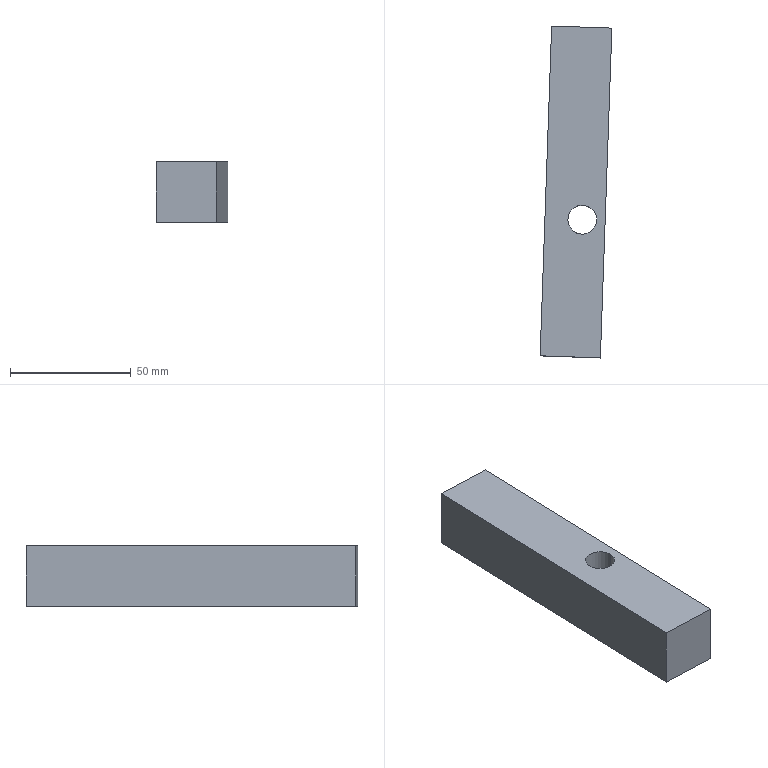Part | STEP file | 1_id1462_x_t | 1 solid | 16 faces | box 29.76 x 137.606 x 25 mm | volume 81885 mm3 | cylinder 6 | plane 6 | cone 4 | commonest cylinder face diameters 5 x4 12 x2
STEP:
#1=CARTESIAN_POINT('',(0.,0.,0.));
#2=DIRECTION('',(0.,0.,1.));
#3=DIRECTION('',(1.,0.,0.));
#4=AXIS2_PLACEMENT_3D('',#1,#2,#3);
#5=CARTESIAN_POINT('',(978.413,154.145,40.46));
#6=VERTEX_POINT('',#5);
#7=CARTESIAN_POINT('',(978.413,154.145,35.46));
#8=VERTEX_POINT('',#7);
#9=CARTESIAN_POINT('',(978.413,154.145,37.96));
#10=DIRECTION('',(0.0349,0.9994,0.));
#11=DIRECTION('',(0.,0.,1.));
#12=AXIS2_PLACEMENT_3D('',#9,#10,#11);
#13=CIRCLE('',#12,2.5);
#14=CARTESIAN_POINT('',(978.389,153.467,37.96));
#15=DIRECTION('',(0.0349,0.9994,0.));
#16=DIRECTION('',(0.,0.,-1.));
#17=AXIS2_PLACEMENT_3D('',#14,#15,#16);
#18=CONICAL_SURFACE('',#17,1.324,1.047);
#19=CARTESIAN_POINT('',(3.142,0.6788));
#20=DIRECTION('',(1.,0.));
#21=VECTOR('',#20,1.);
#22=LINE('',#19,#21);
#23=(GEOMETRIC_REPRESENTATION_CONTEXT(2)PARAMETRIC_REPRESENTATION_CONTEXT()REPRESENTATION_CONTEXT('',''));
#24=DEFINITIONAL_REPRESENTATION('',(#22),#23);
#25=PCURVE('',#18,#24);
#26=CARTESIAN_POINT('',(978.413,154.145,37.96));
#27=DIRECTION('',(-0.0349,-0.9994,0.));
#28=DIRECTION('',(0.,0.,-1.));
#29=AXIS2_PLACEMENT_3D('',#26,#27,#28);
#30=CYLINDRICAL_SURFACE('',#29,2.5);
#31=CARTESIAN_POINT('',(3.142,0.));
#32=DIRECTION('',(-1.,0.));
#33=VECTOR('',#32,1.);
#34=LINE('',#31,#33);
#35=(GEOMETRIC_REPRESENTATION_CONTEXT(2)PARAMETRIC_REPRESENTATION_CONTEXT()REPRESENTATION_CONTEXT('',''));
#36=DEFINITIONAL_REPRESENTATION('',(#34),#35);
#37=PCURVE('',#30,#36);
#38=SURFACE_CURVE('',#13,(#25,#37),.PCURVE_S1.);
#39=EDGE_CURVE('',#6,#8,#38,.T.);
#40=ORIENTED_EDGE('',*,*,#39,.F.);
#41=CARTESIAN_POINT('',(978.362,152.703,37.96));
#42=VERTEX_POINT('',#41);
#43=CARTESIAN_POINT('',(978.362,152.703,37.96));
#44=DIRECTION('',(0.01745,0.4997,0.866));
#45=VECTOR('',#44,1.);
#46=LINE('',#43,#45);
#47=CARTESIAN_POINT('',(3.142,-0.7646));
#48=CARTESIAN_POINT('',(3.142,-0.7427));
#49=CARTESIAN_POINT('',(3.142,-0.699));
#50=CARTESIAN_POINT('',(3.142,-0.6334));
#51=CARTESIAN_POINT('',(3.142,-0.5678));
#52=CARTESIAN_POINT('',(3.142,-0.5022));
#53=CARTESIAN_POINT('',(3.142,-0.4365));
#54=CARTESIAN_POINT('',(3.142,-0.3709));
#55=CARTESIAN_POINT('',(3.142,-0.3053));
#56=CARTESIAN_POINT('',(3.142,-0.2397));
#57=CARTESIAN_POINT('',(3.142,-0.1741));
#58=CARTESIAN_POINT('',(3.142,-0.1085));
#59=CARTESIAN_POINT('',(3.142,-0.0429));
#60=CARTESIAN_POINT('',(3.142,0.02271));
#61=CARTESIAN_POINT('',(3.142,0.08832));
#62=CARTESIAN_POINT('',(3.142,0.1539));
#63=CARTESIAN_POINT('',(3.142,0.2195));
#64=CARTESIAN_POINT('',(3.142,0.2851));
#65=CARTESIAN_POINT('',(3.142,0.3508));
#66=CARTESIAN_POINT('',(3.142,0.4164));
#67=CARTESIAN_POINT('',(3.142,0.482));
#68=CARTESIAN_POINT('',(3.142,0.5476));
#69=CARTESIAN_POINT('',(3.142,0.6132));
#70=CARTESIAN_POINT('',(3.142,0.6569));
#71=CARTESIAN_POINT('',(3.142,0.6788));
#72=B_SPLINE_CURVE_WITH_KNOTS('',3,(#47,#48,#49,#50,#51,#52,#53,#54,#55,#56,#57,#58,#59,#60,#61,#62,#63,#64,#65,#66,#67,#68,#69,#70,#71),.UNSPECIFIED.,.F.,.F.,(4,1,1,1,1,1,1,1,1,1,1,1,1,1,1,1,1,1,1,1,1,1,4),(0.,0.1312,0.2624,0.3936,0.5249,0.6561,0.7873,0.9185,1.05,1.181,1.312,1.443,1.575,1.706,1.837,1.968,2.099,2.231,2.362,2.493,2.624,2.756,2.887),.QUASI_UNIFORM_KNOTS.);
#73=(GEOMETRIC_REPRESENTATION_CONTEXT(2)PARAMETRIC_REPRESENTATION_CONTEXT()REPRESENTATION_CONTEXT('',''));
#74=DEFINITIONAL_REPRESENTATION('',(#72),#73);
#75=PCURVE('',#18,#74);
#76=CARTESIAN_POINT('',(978.389,153.467,37.96));
#77=DIRECTION('',(0.0349,0.9994,0.));
#78=DIRECTION('',(0.,0.,-1.));
#79=AXIS2_PLACEMENT_3D('',#76,#77,#78);
#80=CONICAL_SURFACE('',#79,1.324,1.047);
#81=CARTESIAN_POINT('',(3.142,-0.7646));
#82=CARTESIAN_POINT('',(3.142,-0.7427));
#83=CARTESIAN_POINT('',(3.142,-0.699));
#84=CARTESIAN_POINT('',(3.142,-0.6334));
#85=CARTESIAN_POINT('',(3.142,-0.5678));
#86=CARTESIAN_POINT('',(3.142,-0.5022));
#87=CARTESIAN_POINT('',(3.142,-0.4365));
#88=CARTESIAN_POINT('',(3.142,-0.3709));
#89=CARTESIAN_POINT('',(3.142,-0.3053));
#90=CARTESIAN_POINT('',(3.142,-0.2397));
#91=CARTESIAN_POINT('',(3.142,-0.1741));
#92=CARTESIAN_POINT('',(3.142,-0.1085));
#93=CARTESIAN_POINT('',(3.142,-0.0429));
#94=CARTESIAN_POINT('',(3.142,0.02271));
#95=CARTESIAN_POINT('',(3.142,0.08832));
#96=CARTESIAN_POINT('',(3.142,0.1539));
#97=CARTESIAN_POINT('',(3.142,0.2195));
#98=CARTESIAN_POINT('',(3.142,0.2851));
#99=CARTESIAN_POINT('',(3.142,0.3508));
#100=CARTESIAN_POINT('',(3.142,0.4164));
#101=CARTESIAN_POINT('',(3.142,0.482));
#102=CARTESIAN_POINT('',(3.142,0.5476));
#103=CARTESIAN_POINT('',(3.142,0.6132));
#104=CARTESIAN_POINT('',(3.142,0.6569));
#105=CARTESIAN_POINT('',(3.142,0.6788));
#106=B_SPLINE_CURVE_WITH_KNOTS('',3,(#81,#82,#83,#84,#85,#86,#87,#88,#89,#90,#91,#92,#93,#94,#95,#96,#97,#98,#99,#100,#101,#102,#103,#104,#105),.UNSPECIFIED.,.F.,.F.,(4,1,1,1,1,1,1,1,1,1,1,1,1,1,1,1,1,1,1,1,1,1,4),(0.,0.1312,0.2624,0.3936,0.5249,0.6561,0.7873,0.9185,1.05,1.181,1.312,1.443,1.575,1.706,1.837,1.968,2.099,2.231,2.362,2.493,2.624,2.756,2.887),.QUASI_UNIFORM_KNOTS.);
#107=(GEOMETRIC_REPRESENTATION_CONTEXT(2)PARAMETRIC_REPRESENTATION_CONTEXT()REPRESENTATION_CONTEXT('',''));
#108=DEFINITIONAL_REPRESENTATION('',(#106),#107);
#109=PCURVE('',#80,#108);
#110=SURFACE_CURVE('',#46,(#75,#109),.PCURVE_S1.);
#111=EDGE_CURVE('',#42,#6,#110,.T.);
#112=ORIENTED_EDGE('',*,*,#111,.F.);
#113=CARTESIAN_POINT('',(978.362,152.703,37.96));
#114=DIRECTION('',(-0.01745,-0.4997,0.866));
#115=VECTOR('',#114,1.);
#116=LINE('',#113,#115);
#117=CARTESIAN_POINT('',(6.283,0.6788));
#118=CARTESIAN_POINT('',(6.283,0.6569));
#119=CARTESIAN_POINT('',(6.283,0.6132));
#120=CARTESIAN_POINT('',(6.283,0.5476));
#121=CARTESIAN_POINT('',(6.283,0.482));
#122=CARTESIAN_POINT('',(6.283,0.4164));
#123=CARTESIAN_POINT('',(6.283,0.3508));
#124=CARTESIAN_POINT('',(6.283,0.2851));
#125=CARTESIAN_POINT('',(6.283,0.2195));
#126=CARTESIAN_POINT('',(6.283,0.1539));
#127=CARTESIAN_POINT('',(6.283,0.08832));
#128=CARTESIAN_POINT('',(6.283,0.02271));
#129=CARTESIAN_POINT('',(6.283,-0.0429));
#130=CARTESIAN_POINT('',(6.283,-0.1085));
#131=CARTESIAN_POINT('',(6.283,-0.1741));
#132=CARTESIAN_POINT('',(6.283,-0.2397));
#133=CARTESIAN_POINT('',(6.283,-0.3053));
#134=CARTESIAN_POINT('',(6.283,-0.3709));
#135=CARTESIAN_POINT('',(6.283,-0.4365));
#136=CARTESIAN_POINT('',(6.283,-0.5022));
#137=CARTESIAN_POINT('',(6.283,-0.5678));
#138=CARTESIAN_POINT('',(6.283,-0.6334));
#139=CARTESIAN_POINT('',(6.283,-0.699));
#140=CARTESIAN_POINT('',(6.283,-0.7427));
#141=CARTESIAN_POINT('',(6.283,-0.7646));
#142=B_SPLINE_CURVE_WITH_KNOTS('',3,(#117,#118,#119,#120,#121,#122,#123,#124,#125,#126,#127,#128,#129,#130,#131,#132,#133,#134,#135,#136,#137,#138,#139,#140,#141),.UNSPECIFIED.,.F.,.F.,(4,1,1,1,1,1,1,1,1,1,1,1,1,1,1,1,1,1,1,1,1,1,4),(-2.887,-2.756,-2.624,-2.493,-2.362,-2.231,-2.099,-1.968,-1.837,-1.706,-1.575,-1.443,-1.312,-1.181,-1.05,-0.9185,-0.7873,-0.6561,-0.5249,-0.3936,-0.2624,-0.1312,0.),.QUASI_UNIFORM_KNOTS.);
#143=(GEOMETRIC_REPRESENTATION_CONTEXT(2)PARAMETRIC_REPRESENTATION_CONTEXT()REPRESENTATION_CONTEXT('',''));
#144=DEFINITIONAL_REPRESENTATION('',(#142),#143);
#145=PCURVE('',#18,#144);
#146=CARTESIAN_POINT('',(0.,0.6788));
#147=CARTESIAN_POINT('',(0.,0.6569));
#148=CARTESIAN_POINT('',(0.,0.6132));
#149=CARTESIAN_POINT('',(0.,0.5476));
#150=CARTESIAN_POINT('',(0.,0.482));
#151=CARTESIAN_POINT('',(0.,0.4164));
#152=CARTESIAN_POINT('',(0.,0.3508));
#153=CARTESIAN_POINT('',(0.,0.2851));
#154=CARTESIAN_POINT('',(0.,0.2195));
#155=CARTESIAN_POINT('',(0.,0.1539));
#156=CARTESIAN_POINT('',(0.,0.08832));
#157=CARTESIAN_POINT('',(0.,0.02271));
#158=CARTESIAN_POINT('',(0.,-0.0429));
#159=CARTESIAN_POINT('',(0.,-0.1085));
#160=CARTESIAN_POINT('',(0.,-0.1741));
#161=CARTESIAN_POINT('',(0.,-0.2397));
#162=CARTESIAN_POINT('',(0.,-0.3053));
#163=CARTESIAN_POINT('',(0.,-0.3709));
#164=CARTESIAN_POINT('',(0.,-0.4365));
#165=CARTESIAN_POINT('',(0.,-0.5022));
#166=CARTESIAN_POINT('',(0.,-0.5678));
#167=CARTESIAN_POINT('',(0.,-0.6334));
#168=CARTESIAN_POINT('',(0.,-0.699));
#169=CARTESIAN_POINT('',(0.,-0.7427));
#170=CARTESIAN_POINT('',(0.,-0.7646));
#171=B_SPLINE_CURVE_WITH_KNOTS('',3,(#146,#147,#148,#149,#150,#151,#152,#153,#154,#155,#156,#157,#158,#159,#160,#161,#162,#163,#164,#165,#166,#167,#168,#169,#170),.UNSPECIFIED.,.F.,.F.,(4,1,1,1,1,1,1,1,1,1,1,1,1,1,1,1,1,1,1,1,1,1,4),(-2.887,-2.756,-2.624,-2.493,-2.362,-2.231,-2.099,-1.968,-1.837,-1.706,-1.575,-1.443,-1.312,-1.181,-1.05,-0.9185,-0.7873,-0.6561,-0.5249,-0.3936,-0.2624,-0.1312,0.),.QUASI_UNIFORM_KNOTS.);
#172=(GEOMETRIC_REPRESENTATION_CONTEXT(2)PARAMETRIC_REPRESENTATION_CONTEXT()REPRESENTATION_CONTEXT('',''));
#173=DEFINITIONAL_REPRESENTATION('',(#171),#172);
#174=PCURVE('',#80,#173);
#175=SURFACE_CURVE('',#116,(#145,#174),.PCURVE_S1.);
#176=EDGE_CURVE('',#8,#42,#175,.T.);
#177=ORIENTED_EDGE('',*,*,#176,.F.);
#178=EDGE_LOOP('',(#40,#112,#177));
#179=FACE_BOUND('',#178,.F.);
#180=ADVANCED_FACE('',(#179),#18,.F.);
#181=ORIENTED_EDGE('',*,*,#39,.T.);
#182=CARTESIAN_POINT('',(979.105,173.959,35.46));
#183=VERTEX_POINT('',#182);
#184=CARTESIAN_POINT('',(979.105,173.959,35.46));
#185=DIRECTION('',(0.0349,0.9994,0.));
#186=VECTOR('',#185,1.);
#187=LINE('',#184,#186);
#188=CARTESIAN_POINT('',(0.,-19.826));
#189=DIRECTION('',(0.,-1.));
#190=VECTOR('',#189,1.);
#191=LINE('',#188,#190);
#192=(GEOMETRIC_REPRESENTATION_CONTEXT(2)PARAMETRIC_REPRESENTATION_CONTEXT()REPRESENTATION_CONTEXT('',''));
#193=DEFINITIONAL_REPRESENTATION('',(#191),#192);
#194=PCURVE('',#30,#193);
#195=CARTESIAN_POINT('',(978.413,154.145,37.96));
#196=DIRECTION('',(-0.0349,-0.9994,0.));
#197=DIRECTION('',(0.,0.,-1.));
#198=AXIS2_PLACEMENT_3D('',#195,#196,#197);
#199=CYLINDRICAL_SURFACE('',#198,2.5);
#200=CARTESIAN_POINT('',(6.283,-19.826));
#201=DIRECTION('',(0.,-1.));
#202=VECTOR('',#201,1.);
#203=LINE('',#200,#202);
#204=(GEOMETRIC_REPRESENTATION_CONTEXT(2)PARAMETRIC_REPRESENTATION_CONTEXT()REPRESENTATION_CONTEXT('',''));
#205=DEFINITIONAL_REPRESENTATION('',(#203),#204);
#206=PCURVE('',#199,#205);
#207=SURFACE_CURVE('',#187,(#194,#206),.PCURVE_S1.);
#208=EDGE_CURVE('',#8,#183,#207,.T.);
#209=ORIENTED_EDGE('',*,*,#208,.T.);
#210=CARTESIAN_POINT('',(979.105,173.959,40.46));
#211=VERTEX_POINT('',#210);
#212=CARTESIAN_POINT('',(979.105,173.959,37.96));
#213=DIRECTION('',(-0.0349,-0.9994,0.));
#214=DIRECTION('',(0.,0.,-1.));
#215=AXIS2_PLACEMENT_3D('',#212,#213,#214);
#216=CIRCLE('',#215,2.5);
#217=CARTESIAN_POINT('',(0.,-19.826));
#218=DIRECTION('',(1.,0.));
#219=VECTOR('',#218,1.);
#220=LINE('',#217,#219);
#221=(GEOMETRIC_REPRESENTATION_CONTEXT(2)PARAMETRIC_REPRESENTATION_CONTEXT()REPRESENTATION_CONTEXT('',''));
#222=DEFINITIONAL_REPRESENTATION('',(#220),#221);
#223=PCURVE('',#30,#222);
#224=CARTESIAN_POINT('',(998.241,173.29,9.388));
#225=DIRECTION('',(-0.0349,-0.9994,0.));
#226=DIRECTION('',(0.,0.,1.));
#227=AXIS2_PLACEMENT_3D('',#224,#225,#226);
#228=PLANE('',#227);
#229=CARTESIAN_POINT('',(28.572,19.148));
#230=DIRECTION('',(-1.,0.));
#231=AXIS2_PLACEMENT_2D('',#229,#230);
#232=CIRCLE('',#231,2.5);
#233=(GEOMETRIC_REPRESENTATION_CONTEXT(2)PARAMETRIC_REPRESENTATION_CONTEXT()REPRESENTATION_CONTEXT('',''));
#234=DEFINITIONAL_REPRESENTATION('',(#232),#233);
#235=PCURVE('',#228,#234);
#236=SURFACE_CURVE('',#216,(#223,#235),.PCURVE_S1.);
#237=EDGE_CURVE('',#183,#211,#236,.T.);
#238=ORIENTED_EDGE('',*,*,#237,.T.);
#239=CARTESIAN_POINT('',(979.105,173.959,40.46));
#240=DIRECTION('',(-0.0349,-0.9994,0.));
#241=VECTOR('',#240,1.);
#242=LINE('',#239,#241);
#243=CARTESIAN_POINT('',(3.142,-19.826));
#244=DIRECTION('',(0.,1.));
#245=VECTOR('',#244,1.);
#246=LINE('',#243,#245);
#247=(GEOMETRIC_REPRESENTATION_CONTEXT(2)PARAMETRIC_REPRESENTATION_CONTEXT()REPRESENTATION_CONTEXT('',''));
#248=DEFINITIONAL_REPRESENTATION('',(#246),#247);
#249=PCURVE('',#30,#248);
#250=CARTESIAN_POINT('',(3.142,-19.826));
#251=DIRECTION('',(0.,1.));
#252=VECTOR('',#251,1.);
#253=LINE('',#250,#252);
#254=(GEOMETRIC_REPRESENTATION_CONTEXT(2)PARAMETRIC_REPRESENTATION_CONTEXT()REPRESENTATION_CONTEXT('',''));
#255=DEFINITIONAL_REPRESENTATION('',(#253),#254);
#256=PCURVE('',#199,#255);
#257=SURFACE_CURVE('',#242,(#249,#256),.PCURVE_S1.);
#258=EDGE_CURVE('',#211,#6,#257,.T.);
#259=ORIENTED_EDGE('',*,*,#258,.T.);
#260=EDGE_LOOP('',(#181,#209,#238,#259));
#261=FACE_BOUND('',#260,.F.);
#262=ADVANCED_FACE('',(#261),#30,.F.);
#263=CARTESIAN_POINT('',(978.413,154.145,37.96));
#264=DIRECTION('',(0.0349,0.9994,0.));
#265=DIRECTION('',(0.,0.,-1.));
#266=AXIS2_PLACEMENT_3D('',#263,#264,#265);
#267=CIRCLE('',#266,2.5);
#268=CARTESIAN_POINT('',(6.283,0.));
#269=DIRECTION('',(-1.,0.));
#270=VECTOR('',#269,1.);
#271=LINE('',#268,#270);
#272=(GEOMETRIC_REPRESENTATION_CONTEXT(2)PARAMETRIC_REPRESENTATION_CONTEXT()REPRESENTATION_CONTEXT('',''));
#273=DEFINITIONAL_REPRESENTATION('',(#271),#272);
#274=PCURVE('',#199,#273);
#275=CARTESIAN_POINT('',(0.,0.6788));
#276=DIRECTION('',(1.,0.));
#277=VECTOR('',#276,1.);
#278=LINE('',#275,#277);
#279=(GEOMETRIC_REPRESENTATION_CONTEXT(2)PARAMETRIC_REPRESENTATION_CONTEXT()REPRESENTATION_CONTEXT('',''));
#280=DEFINITIONAL_REPRESENTATION('',(#278),#279);
#281=PCURVE('',#80,#280);
#282=SURFACE_CURVE('',#267,(#274,#281),.PCURVE_S1.);
#283=EDGE_CURVE('',#8,#6,#282,.T.);
#284=ORIENTED_EDGE('',*,*,#283,.T.);
#285=ORIENTED_EDGE('',*,*,#258,.F.);
#286=CARTESIAN_POINT('',(976.606,174.046,37.96));
#287=VERTEX_POINT('',#286);
#288=CARTESIAN_POINT('',(979.105,173.959,37.96));
#289=DIRECTION('',(-0.0349,-0.9994,0.));
#290=DIRECTION('',(0.,0.,1.));
#291=AXIS2_PLACEMENT_3D('',#288,#289,#290);
#292=CIRCLE('',#291,2.5);
#293=CARTESIAN_POINT('',(3.142,-19.826));
#294=DIRECTION('',(1.,0.));
#295=VECTOR('',#294,1.);
#296=LINE('',#293,#295);
#297=(GEOMETRIC_REPRESENTATION_CONTEXT(2)PARAMETRIC_REPRESENTATION_CONTEXT()REPRESENTATION_CONTEXT('',''));
#298=DEFINITIONAL_REPRESENTATION('',(#296),#297);
#299=PCURVE('',#199,#298);
#300=CARTESIAN_POINT('',(28.572,19.148));
#301=DIRECTION('',(1.,0.));
#302=AXIS2_PLACEMENT_2D('',#300,#301);
#303=CIRCLE('',#302,2.5);
#304=(GEOMETRIC_REPRESENTATION_CONTEXT(2)PARAMETRIC_REPRESENTATION_CONTEXT()REPRESENTATION_CONTEXT('',''));
#305=DEFINITIONAL_REPRESENTATION('',(#303),#304);
#306=PCURVE('',#228,#305);
#307=SURFACE_CURVE('',#292,(#299,#306),.PCURVE_S1.);
#308=EDGE_CURVE('',#211,#287,#307,.T.);
#309=ORIENTED_EDGE('',*,*,#308,.T.);
#310=CARTESIAN_POINT('',(979.105,173.959,37.96));
#311=DIRECTION('',(-0.0349,-0.9994,0.));
#312=DIRECTION('',(-0.9994,0.0349,0.));
#313=AXIS2_PLACEMENT_3D('',#310,#311,#312);
#314=CIRCLE('',#313,2.5);
#315=CARTESIAN_POINT('',(4.712,-19.826));
#316=DIRECTION('',(1.,0.));
#317=VECTOR('',#316,1.);
#318=LINE('',#315,#317);
#319=(GEOMETRIC_REPRESENTATION_CONTEXT(2)PARAMETRIC_REPRESENTATION_CONTEXT()REPRESENTATION_CONTEXT('',''));
#320=DEFINITIONAL_REPRESENTATION('',(#318),#319);
#321=PCURVE('',#199,#320);
#322=CARTESIAN_POINT('',(28.572,19.148));
#323=DIRECTION('',(0.,1.));
#324=AXIS2_PLACEMENT_2D('',#322,#323);
#325=CIRCLE('',#324,2.5);
#326=(GEOMETRIC_REPRESENTATION_CONTEXT(2)PARAMETRIC_REPRESENTATION_CONTEXT()REPRESENTATION_CONTEXT('',''));
#327=DEFINITIONAL_REPRESENTATION('',(#325),#326);
#328=PCURVE('',#228,#327);
#329=SURFACE_CURVE('',#314,(#321,#328),.PCURVE_S1.);
#330=EDGE_CURVE('',#287,#183,#329,.T.);
#331=ORIENTED_EDGE('',*,*,#330,.T.);
#332=ORIENTED_EDGE('',*,*,#208,.F.);
#333=EDGE_LOOP('',(#284,#285,#309,#331,#332));
#334=FACE_BOUND('',#333,.F.);
#335=ADVANCED_FACE('',(#334),#199,.F.);
#336=ORIENTED_EDGE('',*,*,#283,.F.);
#337=ORIENTED_EDGE('',*,*,#176,.T.);
#338=ORIENTED_EDGE('',*,*,#111,.T.);
#339=EDGE_LOOP('',(#336,#337,#338));
#340=FACE_BOUND('',#339,.F.);
#341=ADVANCED_FACE('',(#340),#80,.F.);
#342=CARTESIAN_POINT('',(994.092,173.435,43.96));
#343=VERTEX_POINT('',#342);
#344=CARTESIAN_POINT('',(994.092,173.435,18.96));
#345=VERTEX_POINT('',#344);
#346=CARTESIAN_POINT('',(994.092,173.435,43.96));
#347=DIRECTION('',(0.,0.,-1.));
#348=VECTOR('',#347,1.);
#349=LINE('',#346,#348);
#350=CARTESIAN_POINT('',(34.572,4.151));
#351=DIRECTION('',(-1.,0.));
#352=VECTOR('',#351,1.);
#353=LINE('',#350,#352);
#354=(GEOMETRIC_REPRESENTATION_CONTEXT(2)PARAMETRIC_REPRESENTATION_CONTEXT()REPRESENTATION_CONTEXT('',''));
#355=DEFINITIONAL_REPRESENTATION('',(#353),#354);
#356=PCURVE('',#228,#355);
#357=CARTESIAN_POINT('',(994.029,171.611,28.96));
#358=DIRECTION('',(0.9994,-0.0349,0.));
#359=DIRECTION('',(-0.0349,-0.9994,0.));
#360=AXIS2_PLACEMENT_3D('',#357,#358,#359);
#361=PLANE('',#360);
#362=CARTESIAN_POINT('',(-1.826,-15.));
#363=DIRECTION('',(0.,1.));
#364=VECTOR('',#363,1.);
#365=LINE('',#362,#364);
#366=(GEOMETRIC_REPRESENTATION_CONTEXT(2)PARAMETRIC_REPRESENTATION_CONTEXT()REPRESENTATION_CONTEXT('',''));
#367=DEFINITIONAL_REPRESENTATION('',(#365),#366);
#368=PCURVE('',#361,#367);
#369=SURFACE_CURVE('',#349,(#356,#368),.PCURVE_S1.);
#370=EDGE_CURVE('',#343,#345,#369,.T.);
#371=ORIENTED_EDGE('',*,*,#370,.T.);
#372=CARTESIAN_POINT('',(969.108,174.308,18.96));
#373=VERTEX_POINT('',#372);
#374=CARTESIAN_POINT('',(969.108,174.308,18.96));
#375=DIRECTION('',(0.9994,-0.0349,0.));
#376=VECTOR('',#375,1.);
#377=LINE('',#374,#376);
#378=CARTESIAN_POINT('',(9.572,29.151));
#379=DIRECTION('',(0.,-1.));
#380=VECTOR('',#379,1.);
#381=LINE('',#378,#380);
#382=(GEOMETRIC_REPRESENTATION_CONTEXT(2)PARAMETRIC_REPRESENTATION_CONTEXT()REPRESENTATION_CONTEXT('',''));
#383=DEFINITIONAL_REPRESENTATION('',(#381),#382);
#384=PCURVE('',#228,#383);
#385=CARTESIAN_POINT('',(988.334,151.797,18.96));
#386=DIRECTION('',(0.,0.,1.));
#387=DIRECTION('',(1.,0.,0.));
#388=AXIS2_PLACEMENT_3D('',#385,#386,#387);
#389=PLANE('',#388);
#390=CARTESIAN_POINT('',(-19.226,22.51));
#391=DIRECTION('',(0.9994,-0.0349));
#392=VECTOR('',#391,1.);
#393=LINE('',#390,#392);
#394=(GEOMETRIC_REPRESENTATION_CONTEXT(2)PARAMETRIC_REPRESENTATION_CONTEXT()REPRESENTATION_CONTEXT('',''));
#395=DEFINITIONAL_REPRESENTATION('',(#393),#394);
#396=PCURVE('',#389,#395);
#397=SURFACE_CURVE('',#377,(#384,#396),.PCURVE_S1.);
#398=EDGE_CURVE('',#373,#345,#397,.T.);
#399=ORIENTED_EDGE('',*,*,#398,.F.);
#400=CARTESIAN_POINT('',(969.108,174.308,43.96));
#401=VERTEX_POINT('',#400);
#402=CARTESIAN_POINT('',(969.108,174.308,43.96));
#403=DIRECTION('',(0.,0.,-1.));
#404=VECTOR('',#403,1.);
#405=LINE('',#402,#404);
#406=CARTESIAN_POINT('',(34.572,29.151));
#407=DIRECTION('',(-1.,0.));
#408=VECTOR('',#407,1.);
#409=LINE('',#406,#408);
#410=(GEOMETRIC_REPRESENTATION_CONTEXT(2)PARAMETRIC_REPRESENTATION_CONTEXT()REPRESENTATION_CONTEXT('',''));
#411=DEFINITIONAL_REPRESENTATION('',(#409),#410);
#412=PCURVE('',#228,#411);
#413=CARTESIAN_POINT('',(968.346,152.495,28.96));
#414=DIRECTION('',(-0.9994,0.0349,0.));
#415=DIRECTION('',(0.,0.,1.));
#416=AXIS2_PLACEMENT_3D('',#413,#414,#415);
#417=PLANE('',#416);
#418=CARTESIAN_POINT('',(15.,21.826));
#419=DIRECTION('',(-1.,0.));
#420=VECTOR('',#419,1.);
#421=LINE('',#418,#420);
#422=(GEOMETRIC_REPRESENTATION_CONTEXT(2)PARAMETRIC_REPRESENTATION_CONTEXT()REPRESENTATION_CONTEXT('',''));
#423=DEFINITIONAL_REPRESENTATION('',(#421),#422);
#424=PCURVE('',#417,#423);
#425=SURFACE_CURVE('',#405,(#412,#424),.PCURVE_S1.);
#426=EDGE_CURVE('',#401,#373,#425,.T.);
#427=ORIENTED_EDGE('',*,*,#426,.F.);
#428=CARTESIAN_POINT('',(994.092,173.435,43.96));
#429=DIRECTION('',(-0.9994,0.0349,0.));
#430=VECTOR('',#429,1.);
#431=LINE('',#428,#430);
#432=CARTESIAN_POINT('',(34.572,4.151));
#433=DIRECTION('',(0.,1.));
#434=VECTOR('',#433,1.);
#435=LINE('',#432,#434);
#436=(GEOMETRIC_REPRESENTATION_CONTEXT(2)PARAMETRIC_REPRESENTATION_CONTEXT()REPRESENTATION_CONTEXT('',''));
#437=DEFINITIONAL_REPRESENTATION('',(#435),#436);
#438=PCURVE('',#228,#437);
#439=CARTESIAN_POINT('',(988.334,151.797,43.96));
#440=DIRECTION('',(0.,0.,1.));
#441=DIRECTION('',(1.,0.,0.));
#442=AXIS2_PLACEMENT_3D('',#439,#440,#441);
#443=PLANE('',#442);
#444=CARTESIAN_POINT('',(5.759,21.638));
#445=DIRECTION('',(-0.9994,0.0349));
#446=VECTOR('',#445,1.);
#447=LINE('',#444,#446);
#448=(GEOMETRIC_REPRESENTATION_CONTEXT(2)PARAMETRIC_REPRESENTATION_CONTEXT()REPRESENTATION_CONTEXT('',''));
#449=DEFINITIONAL_REPRESENTATION('',(#447),#448);
#450=PCURVE('',#443,#449);
#451=SURFACE_CURVE('',#431,(#438,#450),.PCURVE_S1.);
#452=EDGE_CURVE('',#343,#401,#451,.T.);
#453=ORIENTED_EDGE('',*,*,#452,.F.);
#454=EDGE_LOOP('',(#371,#399,#427,#453));
#455=FACE_BOUND('',#454,.T.);
#456=ORIENTED_EDGE('',*,*,#237,.T.);
#457=ORIENTED_EDGE('',*,*,#308,.T.);
#458=ORIENTED_EDGE('',*,*,#330,.T.);
#459=EDGE_LOOP('',(#456,#457,#458));
#460=FACE_BOUND('',#459,.T.);
#461=CARTESIAN_POINT('',(979.105,173.959,22.46));
#462=VERTEX_POINT('',#461);
#463=CARTESIAN_POINT('',(979.105,173.959,27.46));
#464=VERTEX_POINT('',#463);
#465=CARTESIAN_POINT('',(979.105,173.959,24.96));
#466=DIRECTION('',(-0.0349,-0.9994,0.));
#467=DIRECTION('',(0.,0.,-1.));
#468=AXIS2_PLACEMENT_3D('',#465,#466,#467);
#469=CIRCLE('',#468,2.5);
#470=CARTESIAN_POINT('',(15.572,19.148));
#471=DIRECTION('',(-1.,0.));
#472=AXIS2_PLACEMENT_2D('',#470,#471);
#473=CIRCLE('',#472,2.5);
#474=(GEOMETRIC_REPRESENTATION_CONTEXT(2)PARAMETRIC_REPRESENTATION_CONTEXT()REPRESENTATION_CONTEXT('',''));
#475=DEFINITIONAL_REPRESENTATION('',(#473),#474);
#476=PCURVE('',#228,#475);
#477=CARTESIAN_POINT('',(978.413,154.145,24.96));
#478=DIRECTION('',(-0.0349,-0.9994,0.));
#479=DIRECTION('',(0.,0.,-1.));
#480=AXIS2_PLACEMENT_3D('',#477,#478,#479);
#481=CYLINDRICAL_SURFACE('',#480,2.5);
#482=CARTESIAN_POINT('',(0.,-19.826));
#483=DIRECTION('',(1.,0.));
#484=VECTOR('',#483,1.);
#485=LINE('',#482,#484);
#486=(GEOMETRIC_REPRESENTATION_CONTEXT(2)PARAMETRIC_REPRESENTATION_CONTEXT()REPRESENTATION_CONTEXT('',''));
#487=DEFINITIONAL_REPRESENTATION('',(#485),#486);
#488=PCURVE('',#481,#487);
#489=SURFACE_CURVE('',#469,(#476,#488),.PCURVE_S1.);
#490=EDGE_CURVE('',#462,#464,#489,.T.);
#491=ORIENTED_EDGE('',*,*,#490,.T.);
#492=CARTESIAN_POINT('',(976.606,174.046,24.96));
#493=VERTEX_POINT('',#492);
#494=CARTESIAN_POINT('',(979.105,173.959,24.96));
#495=DIRECTION('',(-0.0349,-0.9994,0.));
#496=DIRECTION('',(0.,0.,1.));
#497=AXIS2_PLACEMENT_3D('',#494,#495,#496);
#498=CIRCLE('',#497,2.5);
#499=CARTESIAN_POINT('',(15.572,19.148));
#500=DIRECTION('',(1.,0.));
#501=AXIS2_PLACEMENT_2D('',#499,#500);
#502=CIRCLE('',#501,2.5);
#503=(GEOMETRIC_REPRESENTATION_CONTEXT(2)PARAMETRIC_REPRESENTATION_CONTEXT()REPRESENTATION_CONTEXT('',''));
#504=DEFINITIONAL_REPRESENTATION('',(#502),#503);
#505=PCURVE('',#228,#504);
#506=CARTESIAN_POINT('',(978.413,154.145,24.96));
#507=DIRECTION('',(-0.0349,-0.9994,0.));
#508=DIRECTION('',(0.,0.,-1.));
#509=AXIS2_PLACEMENT_3D('',#506,#507,#508);
#510=CYLINDRICAL_SURFACE('',#509,2.5);
#511=CARTESIAN_POINT('',(3.142,-19.826));
#512=DIRECTION('',(1.,0.));
#513=VECTOR('',#512,1.);
#514=LINE('',#511,#513);
#515=(GEOMETRIC_REPRESENTATION_CONTEXT(2)PARAMETRIC_REPRESENTATION_CONTEXT()REPRESENTATION_CONTEXT('',''));
#516=DEFINITIONAL_REPRESENTATION('',(#514),#515);
#517=PCURVE('',#510,#516);
#518=SURFACE_CURVE('',#498,(#505,#517),.PCURVE_S1.);
#519=EDGE_CURVE('',#464,#493,#518,.T.);
#520=ORIENTED_EDGE('',*,*,#519,.T.);
#521=CARTESIAN_POINT('',(979.105,173.959,24.96));
#522=DIRECTION('',(-0.0349,-0.9994,0.));
#523=DIRECTION('',(-0.9994,0.0349,0.));
#524=AXIS2_PLACEMENT_3D('',#521,#522,#523);
#525=CIRCLE('',#524,2.5);
#526=CARTESIAN_POINT('',(15.572,19.148));
#527=DIRECTION('',(0.,1.));
#528=AXIS2_PLACEMENT_2D('',#526,#527);
#529=CIRCLE('',#528,2.5);
#530=(GEOMETRIC_REPRESENTATION_CONTEXT(2)PARAMETRIC_REPRESENTATION_CONTEXT()REPRESENTATION_CONTEXT('',''));
#531=DEFINITIONAL_REPRESENTATION('',(#529),#530);
#532=PCURVE('',#228,#531);
#533=CARTESIAN_POINT('',(4.712,-19.826));
#534=DIRECTION('',(1.,0.));
#535=VECTOR('',#534,1.);
#536=LINE('',#533,#535);
#537=(GEOMETRIC_REPRESENTATION_CONTEXT(2)PARAMETRIC_REPRESENTATION_CONTEXT()REPRESENTATION_CONTEXT('',''));
#538=DEFINITIONAL_REPRESENTATION('',(#536),#537);
#539=PCURVE('',#510,#538);
#540=SURFACE_CURVE('',#525,(#532,#539),.PCURVE_S1.);
#541=EDGE_CURVE('',#493,#462,#540,.T.);
#542=ORIENTED_EDGE('',*,*,#541,.T.);
#543=EDGE_LOOP('',(#491,#520,#542));
#544=FACE_BOUND('',#543,.T.);
#545=ADVANCED_FACE('',(#455,#460,#544),#228,.F.);
#546=CARTESIAN_POINT('',(964.333,37.575,43.96));
#547=VERTEX_POINT('',#546);
#548=CARTESIAN_POINT('',(989.318,36.702,43.96));
#549=VERTEX_POINT('',#548);
#550=CARTESIAN_POINT('',(964.333,37.575,43.96));
#551=DIRECTION('',(0.9994,-0.0349,0.));
#552=VECTOR('',#551,1.);
#553=LINE('',#550,#552);
#554=CARTESIAN_POINT('',(-24.001,-114.223));
#555=DIRECTION('',(0.9994,-0.0349));
#556=VECTOR('',#555,1.);
#557=LINE('',#554,#556);
#558=(GEOMETRIC_REPRESENTATION_CONTEXT(2)PARAMETRIC_REPRESENTATION_CONTEXT()REPRESENTATION_CONTEXT('',''));
#559=DEFINITIONAL_REPRESENTATION('',(#557),#558);
#560=PCURVE('',#443,#559);
#561=CARTESIAN_POINT('',(984.844,36.858,28.96));
#562=DIRECTION('',(-0.0349,-0.9994,0.));
#563=DIRECTION('',(0.,0.,1.));
#564=AXIS2_PLACEMENT_3D('',#561,#562,#563);
#565=PLANE('',#564);
#566=CARTESIAN_POINT('',(15.,20.523));
#567=DIRECTION('',(0.,-1.));
#568=VECTOR('',#567,1.);
#569=LINE('',#566,#568);
#570=(GEOMETRIC_REPRESENTATION_CONTEXT(2)PARAMETRIC_REPRESENTATION_CONTEXT()REPRESENTATION_CONTEXT('',''));
#571=DEFINITIONAL_REPRESENTATION('',(#569),#570);
#572=PCURVE('',#565,#571);
#573=SURFACE_CURVE('',#553,(#560,#572),.PCURVE_S1.);
#574=EDGE_CURVE('',#547,#549,#573,.T.);
#575=ORIENTED_EDGE('',*,*,#574,.T.);
#576=CARTESIAN_POINT('',(989.318,36.702,43.96));
#577=DIRECTION('',(0.0349,0.9994,0.));
#578=VECTOR('',#577,1.);
#579=LINE('',#576,#578);
#580=CARTESIAN_POINT('',(0.9838,-115.095));
#581=DIRECTION('',(0.0349,0.9994));
#582=VECTOR('',#581,1.);
#583=LINE('',#580,#582);
#584=(GEOMETRIC_REPRESENTATION_CONTEXT(2)PARAMETRIC_REPRESENTATION_CONTEXT()REPRESENTATION_CONTEXT('',''));
#585=DEFINITIONAL_REPRESENTATION('',(#583),#584);
#586=PCURVE('',#443,#585);
#587=CARTESIAN_POINT('',(134.991,-15.));
#588=DIRECTION('',(-1.,0.));
#589=VECTOR('',#588,1.);
#590=LINE('',#587,#589);
#591=(GEOMETRIC_REPRESENTATION_CONTEXT(2)PARAMETRIC_REPRESENTATION_CONTEXT()REPRESENTATION_CONTEXT('',''));
#592=DEFINITIONAL_REPRESENTATION('',(#590),#591);
#593=PCURVE('',#361,#592);
#594=SURFACE_CURVE('',#579,(#586,#593),.PCURVE_S1.);
#595=EDGE_CURVE('',#549,#343,#594,.T.);
#596=ORIENTED_EDGE('',*,*,#595,.T.);
#597=ORIENTED_EDGE('',*,*,#452,.T.);
#598=CARTESIAN_POINT('',(969.108,174.308,43.96));
#599=DIRECTION('',(-0.0349,-0.9994,0.));
#600=VECTOR('',#599,1.);
#601=LINE('',#598,#600);
#602=CARTESIAN_POINT('',(-19.226,22.51));
#603=DIRECTION('',(-0.0349,-0.9994));
#604=VECTOR('',#603,1.);
#605=LINE('',#602,#604);
#606=(GEOMETRIC_REPRESENTATION_CONTEXT(2)PARAMETRIC_REPRESENTATION_CONTEXT()REPRESENTATION_CONTEXT('',''));
#607=DEFINITIONAL_REPRESENTATION('',(#605),#606);
#608=PCURVE('',#443,#607);
#609=CARTESIAN_POINT('',(15.,21.826));
#610=DIRECTION('',(0.,-1.));
#611=VECTOR('',#610,1.);
#612=LINE('',#609,#611);
#613=(GEOMETRIC_REPRESENTATION_CONTEXT(2)PARAMETRIC_REPRESENTATION_CONTEXT()REPRESENTATION_CONTEXT('',''));
#614=DEFINITIONAL_REPRESENTATION('',(#612),#613);
#615=PCURVE('',#417,#614);
#616=SURFACE_CURVE('',#601,(#608,#615),.PCURVE_S1.);
#617=EDGE_CURVE('',#401,#547,#616,.T.);
#618=ORIENTED_EDGE('',*,*,#617,.T.);
#619=EDGE_LOOP('',(#575,#596,#597,#618));
#620=FACE_BOUND('',#619,.T.);
#621=CARTESIAN_POINT('',(987.832,93.789,43.96));
#622=VERTEX_POINT('',#621);
#623=CARTESIAN_POINT('',(975.84,94.208,43.96));
#624=VERTEX_POINT('',#623);
#625=CARTESIAN_POINT('',(981.836,93.998,43.96));
#626=DIRECTION('',(0.,0.,-1.));
#627=DIRECTION('',(0.9994,-0.0349,0.));
#628=AXIS2_PLACEMENT_3D('',#625,#626,#627);
#629=CIRCLE('',#628,6.);
#630=CARTESIAN_POINT('',(-0.5013,-58.009));
#631=CARTESIAN_POINT('',(-0.864,-68.395));
#632=CARTESIAN_POINT('',(-9.677,-62.888));
#633=CARTESIAN_POINT('',(-18.49,-57.381));
#634=CARTESIAN_POINT('',(-9.314,-52.502));
#635=CARTESIAN_POINT('',(-0.1386,-47.623));
#636=CARTESIAN_POINT('',(-0.5013,-58.009));
#637=(BOUNDED_CURVE()B_SPLINE_CURVE(2,(#630,#631,#632,#633,#634,#635,#636),.UNSPECIFIED.,.T.,.F.)B_SPLINE_CURVE_WITH_KNOTS((1,2,2,2,2,1),(-2.094,0.,2.094,4.189,6.283,8.378),.UNSPECIFIED.)CURVE()GEOMETRIC_REPRESENTATION_ITEM()RATIONAL_B_SPLINE_CURVE((1.,0.5,1.,0.5,1.,0.5,1.))REPRESENTATION_ITEM(''));
#638=(GEOMETRIC_REPRESENTATION_CONTEXT(2)PARAMETRIC_REPRESENTATION_CONTEXT()REPRESENTATION_CONTEXT('',''));
#639=DEFINITIONAL_REPRESENTATION('',(#637),#638);
#640=PCURVE('',#443,#639);
#641=CARTESIAN_POINT('',(981.836,93.998,12.96));
#642=DIRECTION('',(0.,0.,-1.));
#643=DIRECTION('',(0.9994,-0.0349,0.));
#644=AXIS2_PLACEMENT_3D('',#641,#642,#643);
#645=CYLINDRICAL_SURFACE('',#644,6.);
#646=CARTESIAN_POINT('',(0.,-31.));
#647=DIRECTION('',(1.,0.));
#648=VECTOR('',#647,1.);
#649=LINE('',#646,#648);
#650=(GEOMETRIC_REPRESENTATION_CONTEXT(2)PARAMETRIC_REPRESENTATION_CONTEXT()REPRESENTATION_CONTEXT('',''));
#651=DEFINITIONAL_REPRESENTATION('',(#649),#650);
#652=PCURVE('',#645,#651);
#653=SURFACE_CURVE('',#629,(#640,#652),.PCURVE_S1.);
#654=EDGE_CURVE('',#622,#624,#653,.T.);
#655=ORIENTED_EDGE('',*,*,#654,.T.);
#656=CARTESIAN_POINT('',(981.836,93.998,43.96));
#657=DIRECTION('',(0.,0.,-1.));
#658=DIRECTION('',(-0.9994,0.0349,0.));
#659=AXIS2_PLACEMENT_3D('',#656,#657,#658);
#660=CIRCLE('',#659,6.);
#661=CARTESIAN_POINT('',(-12.494,-57.59));
#662=CARTESIAN_POINT('',(-12.131,-47.204));
#663=CARTESIAN_POINT('',(-3.318,-52.711));
#664=CARTESIAN_POINT('',(5.495,-58.218));
#665=CARTESIAN_POINT('',(-3.681,-63.097));
#666=CARTESIAN_POINT('',(-12.857,-67.976));
#667=CARTESIAN_POINT('',(-12.494,-57.59));
#668=(BOUNDED_CURVE()B_SPLINE_CURVE(2,(#661,#662,#663,#664,#665,#666,#667),.UNSPECIFIED.,.T.,.F.)B_SPLINE_CURVE_WITH_KNOTS((1,2,2,2,2,1),(-2.094,0.,2.094,4.189,6.283,8.378),.UNSPECIFIED.)CURVE()GEOMETRIC_REPRESENTATION_ITEM()RATIONAL_B_SPLINE_CURVE((1.,0.5,1.,0.5,1.,0.5,1.))REPRESENTATION_ITEM(''));
#669=(GEOMETRIC_REPRESENTATION_CONTEXT(2)PARAMETRIC_REPRESENTATION_CONTEXT()REPRESENTATION_CONTEXT('',''));
#670=DEFINITIONAL_REPRESENTATION('',(#668),#669);
#671=PCURVE('',#443,#670);
#672=CARTESIAN_POINT('',(981.836,93.998,12.96));
#673=DIRECTION('',(0.,0.,-1.));
#674=DIRECTION('',(0.9994,-0.0349,0.));
#675=AXIS2_PLACEMENT_3D('',#672,#673,#674);
#676=CYLINDRICAL_SURFACE('',#675,6.);
#677=CARTESIAN_POINT('',(3.142,-31.));
#678=DIRECTION('',(1.,0.));
#679=VECTOR('',#678,1.);
#680=LINE('',#677,#679);
#681=(GEOMETRIC_REPRESENTATION_CONTEXT(2)PARAMETRIC_REPRESENTATION_CONTEXT()REPRESENTATION_CONTEXT('',''));
#682=DEFINITIONAL_REPRESENTATION('',(#680),#681);
#683=PCURVE('',#676,#682);
#684=SURFACE_CURVE('',#660,(#671,#683),.PCURVE_S1.);
#685=EDGE_CURVE('',#624,#622,#684,.T.);
#686=ORIENTED_EDGE('',*,*,#685,.T.);
#687=EDGE_LOOP('',(#655,#686));
#688=FACE_BOUND('',#687,.T.);
#689=ADVANCED_FACE('',(#620,#688),#443,.T.);
#690=ORIENTED_EDGE('',*,*,#617,.F.);
#691=ORIENTED_EDGE('',*,*,#426,.T.);
#692=CARTESIAN_POINT('',(964.333,37.575,18.96));
#693=VERTEX_POINT('',#692);
#694=CARTESIAN_POINT('',(964.333,37.575,18.96));
#695=DIRECTION('',(0.0349,0.9994,0.));
#696=VECTOR('',#695,1.);
#697=LINE('',#694,#696);
#698=CARTESIAN_POINT('',(-10.,-114.991));
#699=DIRECTION('',(0.,1.));
#700=VECTOR('',#699,1.);
#701=LINE('',#698,#700);
#702=(GEOMETRIC_REPRESENTATION_CONTEXT(2)PARAMETRIC_REPRESENTATION_CONTEXT()REPRESENTATION_CONTEXT('',''));
#703=DEFINITIONAL_REPRESENTATION('',(#701),#702);
#704=PCURVE('',#417,#703);
#705=CARTESIAN_POINT('',(-24.001,-114.223));
#706=DIRECTION('',(0.0349,0.9994));
#707=VECTOR('',#706,1.);
#708=LINE('',#705,#707);
#709=(GEOMETRIC_REPRESENTATION_CONTEXT(2)PARAMETRIC_REPRESENTATION_CONTEXT()REPRESENTATION_CONTEXT('',''));
#710=DEFINITIONAL_REPRESENTATION('',(#708),#709);
#711=PCURVE('',#389,#710);
#712=SURFACE_CURVE('',#697,(#704,#711),.PCURVE_S1.);
#713=EDGE_CURVE('',#693,#373,#712,.T.);
#714=ORIENTED_EDGE('',*,*,#713,.F.);
#715=CARTESIAN_POINT('',(964.333,37.575,43.96));
#716=DIRECTION('',(0.,0.,-1.));
#717=VECTOR('',#716,1.);
#718=LINE('',#715,#717);
#719=CARTESIAN_POINT('',(15.,-114.991));
#720=DIRECTION('',(-1.,0.));
#721=VECTOR('',#720,1.);
#722=LINE('',#719,#721);
#723=(GEOMETRIC_REPRESENTATION_CONTEXT(2)PARAMETRIC_REPRESENTATION_CONTEXT()REPRESENTATION_CONTEXT('',''));
#724=DEFINITIONAL_REPRESENTATION('',(#722),#723);
#725=PCURVE('',#417,#724);
#726=CARTESIAN_POINT('',(15.,20.523));
#727=DIRECTION('',(-1.,0.));
#728=VECTOR('',#727,1.);
#729=LINE('',#726,#728);
#730=(GEOMETRIC_REPRESENTATION_CONTEXT(2)PARAMETRIC_REPRESENTATION_CONTEXT()REPRESENTATION_CONTEXT('',''));
#731=DEFINITIONAL_REPRESENTATION('',(#729),#730);
#732=PCURVE('',#565,#731);
#733=SURFACE_CURVE('',#718,(#725,#732),.PCURVE_S1.);
#734=EDGE_CURVE('',#547,#693,#733,.T.);
#735=ORIENTED_EDGE('',*,*,#734,.F.);
#736=EDGE_LOOP('',(#690,#691,#714,#735));
#737=FACE_BOUND('',#736,.T.);
#738=ADVANCED_FACE('',(#737),#417,.T.);
#739=ORIENTED_EDGE('',*,*,#574,.F.);
#740=ORIENTED_EDGE('',*,*,#734,.T.);
#741=CARTESIAN_POINT('',(989.318,36.702,18.96));
#742=VERTEX_POINT('',#741);
#743=CARTESIAN_POINT('',(989.318,36.702,18.96));
#744=DIRECTION('',(-0.9994,0.0349,0.));
#745=VECTOR('',#744,1.);
#746=LINE('',#743,#745);
#747=CARTESIAN_POINT('',(-10.,-4.477));
#748=DIRECTION('',(0.,1.));
#749=VECTOR('',#748,1.);
#750=LINE('',#747,#749);
#751=(GEOMETRIC_REPRESENTATION_CONTEXT(2)PARAMETRIC_REPRESENTATION_CONTEXT()REPRESENTATION_CONTEXT('',''));
#752=DEFINITIONAL_REPRESENTATION('',(#750),#751);
#753=PCURVE('',#565,#752);
#754=CARTESIAN_POINT('',(0.9838,-115.095));
#755=DIRECTION('',(-0.9994,0.0349));
#756=VECTOR('',#755,1.);
#757=LINE('',#754,#756);
#758=(GEOMETRIC_REPRESENTATION_CONTEXT(2)PARAMETRIC_REPRESENTATION_CONTEXT()REPRESENTATION_CONTEXT('',''));
#759=DEFINITIONAL_REPRESENTATION('',(#757),#758);
#760=PCURVE('',#389,#759);
#761=SURFACE_CURVE('',#746,(#753,#760),.PCURVE_S1.);
#762=EDGE_CURVE('',#742,#693,#761,.T.);
#763=ORIENTED_EDGE('',*,*,#762,.F.);
#764=CARTESIAN_POINT('',(989.318,36.702,43.96));
#765=DIRECTION('',(0.,0.,-1.));
#766=VECTOR('',#765,1.);
#767=LINE('',#764,#766);
#768=CARTESIAN_POINT('',(15.,-4.477));
#769=DIRECTION('',(-1.,0.));
#770=VECTOR('',#769,1.);
#771=LINE('',#768,#770);
#772=(GEOMETRIC_REPRESENTATION_CONTEXT(2)PARAMETRIC_REPRESENTATION_CONTEXT()REPRESENTATION_CONTEXT('',''));
#773=DEFINITIONAL_REPRESENTATION('',(#771),#772);
#774=PCURVE('',#565,#773);
#775=CARTESIAN_POINT('',(134.991,-15.));
#776=DIRECTION('',(0.,1.));
#777=VECTOR('',#776,1.);
#778=LINE('',#775,#777);
#779=(GEOMETRIC_REPRESENTATION_CONTEXT(2)PARAMETRIC_REPRESENTATION_CONTEXT()REPRESENTATION_CONTEXT('',''));
#780=DEFINITIONAL_REPRESENTATION('',(#778),#779);
#781=PCURVE('',#361,#780);
#782=SURFACE_CURVE('',#767,(#774,#781),.PCURVE_S1.);
#783=EDGE_CURVE('',#549,#742,#782,.T.);
#784=ORIENTED_EDGE('',*,*,#783,.F.);
#785=EDGE_LOOP('',(#739,#740,#763,#784));
#786=FACE_BOUND('',#785,.T.);
#787=ADVANCED_FACE('',(#786),#565,.T.);
#788=ORIENTED_EDGE('',*,*,#370,.F.);
#789=ORIENTED_EDGE('',*,*,#595,.F.);
#790=ORIENTED_EDGE('',*,*,#783,.T.);
#791=CARTESIAN_POINT('',(994.092,173.435,18.96));
#792=DIRECTION('',(-0.0349,-0.9994,0.));
#793=VECTOR('',#792,1.);
#794=LINE('',#791,#793);
#795=CARTESIAN_POINT('',(-1.826,10.));
#796=DIRECTION('',(1.,0.));
#797=VECTOR('',#796,1.);
#798=LINE('',#795,#797);
#799=(GEOMETRIC_REPRESENTATION_CONTEXT(2)PARAMETRIC_REPRESENTATION_CONTEXT()REPRESENTATION_CONTEXT('',''));
#800=DEFINITIONAL_REPRESENTATION('',(#798),#799);
#801=PCURVE('',#361,#800);
#802=CARTESIAN_POINT('',(5.759,21.638));
#803=DIRECTION('',(-0.0349,-0.9994));
#804=VECTOR('',#803,1.);
#805=LINE('',#802,#804);
#806=(GEOMETRIC_REPRESENTATION_CONTEXT(2)PARAMETRIC_REPRESENTATION_CONTEXT()REPRESENTATION_CONTEXT('',''));
#807=DEFINITIONAL_REPRESENTATION('',(#805),#806);
#808=PCURVE('',#389,#807);
#809=SURFACE_CURVE('',#794,(#801,#808),.PCURVE_S1.);
#810=EDGE_CURVE('',#345,#742,#809,.T.);
#811=ORIENTED_EDGE('',*,*,#810,.F.);
#812=EDGE_LOOP('',(#788,#789,#790,#811));
#813=FACE_BOUND('',#812,.T.);
#814=ADVANCED_FACE('',(#813),#361,.T.);
#815=ORIENTED_EDGE('',*,*,#398,.T.);
#816=ORIENTED_EDGE('',*,*,#810,.T.);
#817=ORIENTED_EDGE('',*,*,#762,.T.);
#818=ORIENTED_EDGE('',*,*,#713,.T.);
#819=EDGE_LOOP('',(#815,#816,#817,#818));
#820=FACE_BOUND('',#819,.T.);
#821=CARTESIAN_POINT('',(987.832,93.789,18.96));
#822=VERTEX_POINT('',#821);
#823=CARTESIAN_POINT('',(975.84,94.208,18.96));
#824=VERTEX_POINT('',#823);
#825=CARTESIAN_POINT('',(981.836,93.998,18.96));
#826=DIRECTION('',(0.,0.,1.));
#827=DIRECTION('',(0.9994,-0.0349,0.));
#828=AXIS2_PLACEMENT_3D('',#825,#826,#827);
#829=CIRCLE('',#828,6.);
#830=CARTESIAN_POINT('',(-6.498,-57.799));
#831=DIRECTION('',(0.9994,-0.0349));
#832=AXIS2_PLACEMENT_2D('',#830,#831);
#833=CIRCLE('',#832,6.);
#834=(GEOMETRIC_REPRESENTATION_CONTEXT(2)PARAMETRIC_REPRESENTATION_CONTEXT()REPRESENTATION_CONTEXT('',''));
#835=DEFINITIONAL_REPRESENTATION('',(#833),#834);
#836=PCURVE('',#389,#835);
#837=CARTESIAN_POINT('',(6.283,-6.));
#838=DIRECTION('',(-1.,0.));
#839=VECTOR('',#838,1.);
#840=LINE('',#837,#839);
#841=(GEOMETRIC_REPRESENTATION_CONTEXT(2)PARAMETRIC_REPRESENTATION_CONTEXT()REPRESENTATION_CONTEXT('',''));
#842=DEFINITIONAL_REPRESENTATION('',(#840),#841);
#843=PCURVE('',#676,#842);
#844=SURFACE_CURVE('',#829,(#836,#843),.PCURVE_S1.);
#845=EDGE_CURVE('',#822,#824,#844,.T.);
#846=ORIENTED_EDGE('',*,*,#845,.T.);
#847=CARTESIAN_POINT('',(975.836,93.998,18.96));
#848=VERTEX_POINT('',#847);
#849=CARTESIAN_POINT('',(981.836,93.998,18.96));
#850=DIRECTION('',(0.,0.,1.));
#851=DIRECTION('',(-0.9994,0.0349,0.));
#852=AXIS2_PLACEMENT_3D('',#849,#850,#851);
#853=CIRCLE('',#852,6.);
#854=CARTESIAN_POINT('',(-6.498,-57.799));
#855=DIRECTION('',(-0.9994,0.0349));
#856=AXIS2_PLACEMENT_2D('',#854,#855);
#857=CIRCLE('',#856,6.);
#858=(GEOMETRIC_REPRESENTATION_CONTEXT(2)PARAMETRIC_REPRESENTATION_CONTEXT()REPRESENTATION_CONTEXT('',''));
#859=DEFINITIONAL_REPRESENTATION('',(#857),#858);
#860=PCURVE('',#389,#859);
#861=CARTESIAN_POINT('',(3.142,-6.));
#862=DIRECTION('',(-1.,0.));
#863=VECTOR('',#862,1.);
#864=LINE('',#861,#863);
#865=(GEOMETRIC_REPRESENTATION_CONTEXT(2)PARAMETRIC_REPRESENTATION_CONTEXT()REPRESENTATION_CONTEXT('',''));
#866=DEFINITIONAL_REPRESENTATION('',(#864),#865);
#867=PCURVE('',#645,#866);
#868=SURFACE_CURVE('',#853,(#860,#867),.PCURVE_S1.);
#869=EDGE_CURVE('',#824,#848,#868,.T.);
#870=ORIENTED_EDGE('',*,*,#869,.T.);
#871=CARTESIAN_POINT('',(981.836,93.998,18.96));
#872=DIRECTION('',(0.,0.,1.));
#873=DIRECTION('',(-1.,0.,0.));
#874=AXIS2_PLACEMENT_3D('',#871,#872,#873);
#875=CIRCLE('',#874,6.);
#876=CARTESIAN_POINT('',(-6.498,-57.799));
#877=DIRECTION('',(-1.,0.));
#878=AXIS2_PLACEMENT_2D('',#876,#877);
#879=CIRCLE('',#878,6.);
#880=(GEOMETRIC_REPRESENTATION_CONTEXT(2)PARAMETRIC_REPRESENTATION_CONTEXT()REPRESENTATION_CONTEXT('',''));
#881=DEFINITIONAL_REPRESENTATION('',(#879),#880);
#882=PCURVE('',#389,#881);
#883=CARTESIAN_POINT('',(3.107,-6.));
#884=DIRECTION('',(-1.,0.));
#885=VECTOR('',#884,1.);
#886=LINE('',#883,#885);
#887=(GEOMETRIC_REPRESENTATION_CONTEXT(2)PARAMETRIC_REPRESENTATION_CONTEXT()REPRESENTATION_CONTEXT('',''));
#888=DEFINITIONAL_REPRESENTATION('',(#886),#887);
#889=PCURVE('',#645,#888);
#890=SURFACE_CURVE('',#875,(#882,#889),.PCURVE_S1.);
#891=EDGE_CURVE('',#848,#822,#890,.T.);
#892=ORIENTED_EDGE('',*,*,#891,.T.);
#893=EDGE_LOOP('',(#846,#870,#892));
#894=FACE_BOUND('',#893,.T.);
#895=ADVANCED_FACE('',(#820,#894),#389,.F.);
#896=ORIENTED_EDGE('',*,*,#869,.T.);
#897=ORIENTED_EDGE('',*,*,#891,.T.);
#898=CARTESIAN_POINT('',(987.832,93.789,43.96));
#899=DIRECTION('',(0.,0.,-1.));
#900=VECTOR('',#899,1.);
#901=LINE('',#898,#900);
#902=CARTESIAN_POINT('',(0.,-31.));
#903=DIRECTION('',(0.,1.));
#904=VECTOR('',#903,1.);
#905=LINE('',#902,#904);
#906=(GEOMETRIC_REPRESENTATION_CONTEXT(2)PARAMETRIC_REPRESENTATION_CONTEXT()REPRESENTATION_CONTEXT('',''));
#907=DEFINITIONAL_REPRESENTATION('',(#905),#906);
#908=PCURVE('',#645,#907);
#909=CARTESIAN_POINT('',(6.283,-31.));
#910=DIRECTION('',(0.,1.));
#911=VECTOR('',#910,1.);
#912=LINE('',#909,#911);
#913=(GEOMETRIC_REPRESENTATION_CONTEXT(2)PARAMETRIC_REPRESENTATION_CONTEXT()REPRESENTATION_CONTEXT('',''));
#914=DEFINITIONAL_REPRESENTATION('',(#912),#913);
#915=PCURVE('',#676,#914);
#916=SURFACE_CURVE('',#901,(#908,#915),.PCURVE_S1.);
#917=EDGE_CURVE('',#622,#822,#916,.T.);
#918=ORIENTED_EDGE('',*,*,#917,.F.);
#919=ORIENTED_EDGE('',*,*,#654,.T.);
#920=CARTESIAN_POINT('',(975.84,94.208,43.96));
#921=DIRECTION('',(0.,0.,1.));
#922=VECTOR('',#921,1.);
#923=LINE('',#920,#922);
#924=CARTESIAN_POINT('',(3.142,-31.));
#925=DIRECTION('',(0.,-1.));
#926=VECTOR('',#925,1.);
#927=LINE('',#924,#926);
#928=(GEOMETRIC_REPRESENTATION_CONTEXT(2)PARAMETRIC_REPRESENTATION_CONTEXT()REPRESENTATION_CONTEXT('',''));
#929=DEFINITIONAL_REPRESENTATION('',(#927),#928);
#930=PCURVE('',#645,#929);
#931=CARTESIAN_POINT('',(3.142,-31.));
#932=DIRECTION('',(0.,-1.));
#933=VECTOR('',#932,1.);
#934=LINE('',#931,#933);
#935=(GEOMETRIC_REPRESENTATION_CONTEXT(2)PARAMETRIC_REPRESENTATION_CONTEXT()REPRESENTATION_CONTEXT('',''));
#936=DEFINITIONAL_REPRESENTATION('',(#934),#935);
#937=PCURVE('',#676,#936);
#938=SURFACE_CURVE('',#923,(#930,#937),.PCURVE_S1.);
#939=EDGE_CURVE('',#824,#624,#938,.T.);
#940=ORIENTED_EDGE('',*,*,#939,.F.);
#941=EDGE_LOOP('',(#896,#897,#918,#919,#940));
#942=FACE_BOUND('',#941,.F.);
#943=ADVANCED_FACE('',(#942),#645,.F.);
#944=ORIENTED_EDGE('',*,*,#845,.T.);
#945=ORIENTED_EDGE('',*,*,#939,.T.);
#946=ORIENTED_EDGE('',*,*,#685,.T.);
#947=ORIENTED_EDGE('',*,*,#917,.T.);
#948=EDGE_LOOP('',(#944,#945,#946,#947));
#949=FACE_BOUND('',#948,.F.);
#950=ADVANCED_FACE('',(#949),#676,.F.);
#951=CARTESIAN_POINT('',(978.413,154.145,22.46));
#952=VERTEX_POINT('',#951);
#953=CARTESIAN_POINT('',(978.413,154.145,27.46));
#954=VERTEX_POINT('',#953);
#955=CARTESIAN_POINT('',(978.413,154.145,24.96));
#956=DIRECTION('',(0.0349,0.9994,0.));
#957=DIRECTION('',(0.,0.,-1.));
#958=AXIS2_PLACEMENT_3D('',#955,#956,#957);
#959=CIRCLE('',#958,2.5);
#960=CARTESIAN_POINT('',(6.283,0.));
#961=DIRECTION('',(-1.,0.));
#962=VECTOR('',#961,1.);
#963=LINE('',#960,#962);
#964=(GEOMETRIC_REPRESENTATION_CONTEXT(2)PARAMETRIC_REPRESENTATION_CONTEXT()REPRESENTATION_CONTEXT('',''));
#965=DEFINITIONAL_REPRESENTATION('',(#963),#964);
#966=PCURVE('',#510,#965);
#967=CARTESIAN_POINT('',(978.389,153.467,24.96));
#968=DIRECTION('',(0.0349,0.9994,0.));
#969=DIRECTION('',(0.,0.,-1.));
#970=AXIS2_PLACEMENT_3D('',#967,#968,#969);
#971=CONICAL_SURFACE('',#970,1.324,1.047);
#972=CARTESIAN_POINT('',(0.,0.6788));
#973=DIRECTION('',(1.,0.));
#974=VECTOR('',#973,1.);
#975=LINE('',#972,#974);
#976=(GEOMETRIC_REPRESENTATION_CONTEXT(2)PARAMETRIC_REPRESENTATION_CONTEXT()REPRESENTATION_CONTEXT('',''));
#977=DEFINITIONAL_REPRESENTATION('',(#975),#976);
#978=PCURVE('',#971,#977);
#979=SURFACE_CURVE('',#959,(#966,#978),.PCURVE_S1.);
#980=EDGE_CURVE('',#952,#954,#979,.T.);
#981=ORIENTED_EDGE('',*,*,#980,.T.);
#982=CARTESIAN_POINT('',(979.105,173.959,27.46));
#983=DIRECTION('',(0.0349,0.9994,0.));
#984=VECTOR('',#983,1.);
#985=LINE('',#982,#984);
#986=CARTESIAN_POINT('',(3.142,-19.826));
#987=DIRECTION('',(0.,-1.));
#988=VECTOR('',#987,1.);
#989=LINE('',#986,#988);
#990=(GEOMETRIC_REPRESENTATION_CONTEXT(2)PARAMETRIC_REPRESENTATION_CONTEXT()REPRESENTATION_CONTEXT('',''));
#991=DEFINITIONAL_REPRESENTATION('',(#989),#990);
#992=PCURVE('',#510,#991);
#993=CARTESIAN_POINT('',(3.142,-19.826));
#994=DIRECTION('',(0.,-1.));
#995=VECTOR('',#994,1.);
#996=LINE('',#993,#995);
#997=(GEOMETRIC_REPRESENTATION_CONTEXT(2)PARAMETRIC_REPRESENTATION_CONTEXT()REPRESENTATION_CONTEXT('',''));
#998=DEFINITIONAL_REPRESENTATION('',(#996),#997);
#999=PCURVE('',#481,#998);
#1000=SURFACE_CURVE('',#985,(#992,#999),.PCURVE_S1.);
#1001=EDGE_CURVE('',#954,#464,#1000,.T.);
#1002=ORIENTED_EDGE('',*,*,#1001,.T.);
#1003=ORIENTED_EDGE('',*,*,#519,.T.);
#1004=ORIENTED_EDGE('',*,*,#541,.T.);
#1005=CARTESIAN_POINT('',(979.105,173.959,22.46));
#1006=DIRECTION('',(-0.0349,-0.9994,0.));
#1007=VECTOR('',#1006,1.);
#1008=LINE('',#1005,#1007);
#1009=CARTESIAN_POINT('',(6.283,-19.826));
#1010=DIRECTION('',(0.,1.));
#1011=VECTOR('',#1010,1.);
#1012=LINE('',#1009,#1011);
#1013=(GEOMETRIC_REPRESENTATION_CONTEXT(2)PARAMETRIC_REPRESENTATION_CONTEXT()REPRESENTATION_CONTEXT('',''));
#1014=DEFINITIONAL_REPRESENTATION('',(#1012),#1013);
#1015=PCURVE('',#510,#1014);
#1016=CARTESIAN_POINT('',(0.,-19.826));
#1017=DIRECTION('',(0.,1.));
#1018=VECTOR('',#1017,1.);
#1019=LINE('',#1016,#1018);
#1020=(GEOMETRIC_REPRESENTATION_CONTEXT(2)PARAMETRIC_REPRESENTATION_CONTEXT()REPRESENTATION_CONTEXT('',''));
#1021=DEFINITIONAL_REPRESENTATION('',(#1019),#1020);
#1022=PCURVE('',#481,#1021);
#1023=SURFACE_CURVE('',#1008,(#1015,#1022),.PCURVE_S1.);
#1024=EDGE_CURVE('',#462,#952,#1023,.T.);
#1025=ORIENTED_EDGE('',*,*,#1024,.T.);
#1026=EDGE_LOOP('',(#981,#1002,#1003,#1004,#1025));
#1027=FACE_BOUND('',#1026,.F.);
#1028=ADVANCED_FACE('',(#1027),#510,.F.);
#1029=ORIENTED_EDGE('',*,*,#980,.F.);
#1030=CARTESIAN_POINT('',(978.362,152.703,24.96));
#1031=VERTEX_POINT('',#1030);
#1032=CARTESIAN_POINT('',(978.362,152.703,24.96));
#1033=DIRECTION('',(-0.01745,-0.4997,0.866));
#1034=VECTOR('',#1033,1.);
#1035=LINE('',#1032,#1034);
#1036=CARTESIAN_POINT('',(0.,0.6788));
#1037=CARTESIAN_POINT('',(0.,0.6569));
#1038=CARTESIAN_POINT('',(0.,0.6132));
#1039=CARTESIAN_POINT('',(0.,0.5476));
#1040=CARTESIAN_POINT('',(0.,0.482));
#1041=CARTESIAN_POINT('',(0.,0.4164));
#1042=CARTESIAN_POINT('',(0.,0.3508));
#1043=CARTESIAN_POINT('',(0.,0.2851));
#1044=CARTESIAN_POINT('',(0.,0.2195));
#1045=CARTESIAN_POINT('',(0.,0.1539));
#1046=CARTESIAN_POINT('',(0.,0.08832));
#1047=CARTESIAN_POINT('',(0.,0.02271));
#1048=CARTESIAN_POINT('',(0.,-0.0429));
#1049=CARTESIAN_POINT('',(0.,-0.1085));
#1050=CARTESIAN_POINT('',(0.,-0.1741));
#1051=CARTESIAN_POINT('',(0.,-0.2397));
#1052=CARTESIAN_POINT('',(0.,-0.3053));
#1053=CARTESIAN_POINT('',(0.,-0.3709));
#1054=CARTESIAN_POINT('',(0.,-0.4365));
#1055=CARTESIAN_POINT('',(0.,-0.5022));
#1056=CARTESIAN_POINT('',(0.,-0.5678));
#1057=CARTESIAN_POINT('',(0.,-0.6334));
#1058=CARTESIAN_POINT('',(0.,-0.699));
#1059=CARTESIAN_POINT('',(0.,-0.7427));
#1060=CARTESIAN_POINT('',(0.,-0.7646));
#1061=B_SPLINE_CURVE_WITH_KNOTS('',3,(#1036,#1037,#1038,#1039,#1040,#1041,#1042,#1043,#1044,#1045,#1046,#1047,#1048,#1049,#1050,#1051,#1052,#1053,#1054,#1055,#1056,#1057,#1058,#1059,#1060),.UNSPECIFIED.,.F.,.F.,(4,1,1,1,1,1,1,1,1,1,1,1,1,1,1,1,1,1,1,1,1,1,4),(-2.887,-2.756,-2.624,-2.493,-2.362,-2.231,-2.099,-1.968,-1.837,-1.706,-1.575,-1.443,-1.312,-1.181,-1.05,-0.9185,-0.7873,-0.6561,-0.5249,-0.3936,-0.2624,-0.1312,0.),.QUASI_UNIFORM_KNOTS.);
#1062=(GEOMETRIC_REPRESENTATION_CONTEXT(2)PARAMETRIC_REPRESENTATION_CONTEXT()REPRESENTATION_CONTEXT('',''));
#1063=DEFINITIONAL_REPRESENTATION('',(#1061),#1062);
#1064=PCURVE('',#971,#1063);
#1065=CARTESIAN_POINT('',(978.389,153.467,24.96));
#1066=DIRECTION('',(0.0349,0.9994,0.));
#1067=DIRECTION('',(0.,0.,-1.));
#1068=AXIS2_PLACEMENT_3D('',#1065,#1066,#1067);
#1069=CONICAL_SURFACE('',#1068,1.324,1.047);
#1070=CARTESIAN_POINT('',(6.283,0.6788));
#1071=CARTESIAN_POINT('',(6.283,0.6569));
#1072=CARTESIAN_POINT('',(6.283,0.6132));
#1073=CARTESIAN_POINT('',(6.283,0.5476));
#1074=CARTESIAN_POINT('',(6.283,0.482));
#1075=CARTESIAN_POINT('',(6.283,0.4164));
#1076=CARTESIAN_POINT('',(6.283,0.3508));
#1077=CARTESIAN_POINT('',(6.283,0.2851));
#1078=CARTESIAN_POINT('',(6.283,0.2195));
#1079=CARTESIAN_POINT('',(6.283,0.1539));
#1080=CARTESIAN_POINT('',(6.283,0.08832));
#1081=CARTESIAN_POINT('',(6.283,0.02271));
#1082=CARTESIAN_POINT('',(6.283,-0.0429));
#1083=CARTESIAN_POINT('',(6.283,-0.1085));
#1084=CARTESIAN_POINT('',(6.283,-0.1741));
#1085=CARTESIAN_POINT('',(6.283,-0.2397));
#1086=CARTESIAN_POINT('',(6.283,-0.3053));
#1087=CARTESIAN_POINT('',(6.283,-0.3709));
#1088=CARTESIAN_POINT('',(6.283,-0.4365));
#1089=CARTESIAN_POINT('',(6.283,-0.5022));
#1090=CARTESIAN_POINT('',(6.283,-0.5678));
#1091=CARTESIAN_POINT('',(6.283,-0.6334));
#1092=CARTESIAN_POINT('',(6.283,-0.699));
#1093=CARTESIAN_POINT('',(6.283,-0.7427));
#1094=CARTESIAN_POINT('',(6.283,-0.7646));
#1095=B_SPLINE_CURVE_WITH_KNOTS('',3,(#1070,#1071,#1072,#1073,#1074,#1075,#1076,#1077,#1078,#1079,#1080,#1081,#1082,#1083,#1084,#1085,#1086,#1087,#1088,#1089,#1090,#1091,#1092,#1093,#1094),.UNSPECIFIED.,.F.,.F.,(4,1,1,1,1,1,1,1,1,1,1,1,1,1,1,1,1,1,1,1,1,1,4),(-2.887,-2.756,-2.624,-2.493,-2.362,-2.231,-2.099,-1.968,-1.837,-1.706,-1.575,-1.443,-1.312,-1.181,-1.05,-0.9185,-0.7873,-0.6561,-0.5249,-0.3936,-0.2624,-0.1312,0.),.QUASI_UNIFORM_KNOTS.);
#1096=(GEOMETRIC_REPRESENTATION_CONTEXT(2)PARAMETRIC_REPRESENTATION_CONTEXT()REPRESENTATION_CONTEXT('',''));
#1097=DEFINITIONAL_REPRESENTATION('',(#1095),#1096);
#1098=PCURVE('',#1069,#1097);
#1099=SURFACE_CURVE('',#1035,(#1064,#1098),.PCURVE_S1.);
#1100=EDGE_CURVE('',#952,#1031,#1099,.T.);
#1101=ORIENTED_EDGE('',*,*,#1100,.T.);
#1102=CARTESIAN_POINT('',(978.362,152.703,24.96));
#1103=DIRECTION('',(0.01745,0.4997,0.866));
#1104=VECTOR('',#1103,1.);
#1105=LINE('',#1102,#1104);
#1106=CARTESIAN_POINT('',(3.142,-0.7646));
#1107=CARTESIAN_POINT('',(3.142,-0.7427));
#1108=CARTESIAN_POINT('',(3.142,-0.699));
#1109=CARTESIAN_POINT('',(3.142,-0.6334));
#1110=CARTESIAN_POINT('',(3.142,-0.5678));
#1111=CARTESIAN_POINT('',(3.142,-0.5022));
#1112=CARTESIAN_POINT('',(3.142,-0.4365));
#1113=CARTESIAN_POINT('',(3.142,-0.3709));
#1114=CARTESIAN_POINT('',(3.142,-0.3053));
#1115=CARTESIAN_POINT('',(3.142,-0.2397));
#1116=CARTESIAN_POINT('',(3.142,-0.1741));
#1117=CARTESIAN_POINT('',(3.142,-0.1085));
#1118=CARTESIAN_POINT('',(3.142,-0.0429));
#1119=CARTESIAN_POINT('',(3.142,0.02271));
#1120=CARTESIAN_POINT('',(3.142,0.08832));
#1121=CARTESIAN_POINT('',(3.142,0.1539));
#1122=CARTESIAN_POINT('',(3.142,0.2195));
#1123=CARTESIAN_POINT('',(3.142,0.2851));
#1124=CARTESIAN_POINT('',(3.142,0.3508));
#1125=CARTESIAN_POINT('',(3.142,0.4164));
#1126=CARTESIAN_POINT('',(3.142,0.482));
#1127=CARTESIAN_POINT('',(3.142,0.5476));
#1128=CARTESIAN_POINT('',(3.142,0.6132));
#1129=CARTESIAN_POINT('',(3.142,0.6569));
#1130=CARTESIAN_POINT('',(3.142,0.6788));
#1131=B_SPLINE_CURVE_WITH_KNOTS('',3,(#1106,#1107,#1108,#1109,#1110,#1111,#1112,#1113,#1114,#1115,#1116,#1117,#1118,#1119,#1120,#1121,#1122,#1123,#1124,#1125,#1126,#1127,#1128,#1129,#1130),.UNSPECIFIED.,.F.,.F.,(4,1,1,1,1,1,1,1,1,1,1,1,1,1,1,1,1,1,1,1,1,1,4),(0.,0.1312,0.2624,0.3936,0.5249,0.6561,0.7873,0.9185,1.05,1.181,1.312,1.443,1.575,1.706,1.837,1.968,2.099,2.231,2.362,2.493,2.624,2.756,2.887),.QUASI_UNIFORM_KNOTS.);
#1132=(GEOMETRIC_REPRESENTATION_CONTEXT(2)PARAMETRIC_REPRESENTATION_CONTEXT()REPRESENTATION_CONTEXT('',''));
#1133=DEFINITIONAL_REPRESENTATION('',(#1131),#1132);
#1134=PCURVE('',#971,#1133);
#1135=CARTESIAN_POINT('',(3.142,-0.7646));
#1136=CARTESIAN_POINT('',(3.142,-0.7427));
#1137=CARTESIAN_POINT('',(3.142,-0.699));
#1138=CARTESIAN_POINT('',(3.142,-0.6334));
#1139=CARTESIAN_POINT('',(3.142,-0.5678));
#1140=CARTESIAN_POINT('',(3.142,-0.5022));
#1141=CARTESIAN_POINT('',(3.142,-0.4365));
#1142=CARTESIAN_POINT('',(3.142,-0.3709));
#1143=CARTESIAN_POINT('',(3.142,-0.3053));
#1144=CARTESIAN_POINT('',(3.142,-0.2397));
#1145=CARTESIAN_POINT('',(3.142,-0.1741));
#1146=CARTESIAN_POINT('',(3.142,-0.1085));
#1147=CARTESIAN_POINT('',(3.142,-0.0429));
#1148=CARTESIAN_POINT('',(3.142,0.02271));
#1149=CARTESIAN_POINT('',(3.142,0.08832));
#1150=CARTESIAN_POINT('',(3.142,0.1539));
#1151=CARTESIAN_POINT('',(3.142,0.2195));
#1152=CARTESIAN_POINT('',(3.142,0.2851));
#1153=CARTESIAN_POINT('',(3.142,0.3508));
#1154=CARTESIAN_POINT('',(3.142,0.4164));
#1155=CARTESIAN_POINT('',(3.142,0.482));
#1156=CARTESIAN_POINT('',(3.142,0.5476));
#1157=CARTESIAN_POINT('',(3.142,0.6132));
#1158=CARTESIAN_POINT('',(3.142,0.6569));
#1159=CARTESIAN_POINT('',(3.142,0.6788));
#1160=B_SPLINE_CURVE_WITH_KNOTS('',3,(#1135,#1136,#1137,#1138,#1139,#1140,#1141,#1142,#1143,#1144,#1145,#1146,#1147,#1148,#1149,#1150,#1151,#1152,#1153,#1154,#1155,#1156,#1157,#1158,#1159),.UNSPECIFIED.,.F.,.F.,(4,1,1,1,1,1,1,1,1,1,1,1,1,1,1,1,1,1,1,1,1,1,4),(0.,0.1312,0.2624,0.3936,0.5249,0.6561,0.7873,0.9185,1.05,1.181,1.312,1.443,1.575,1.706,1.837,1.968,2.099,2.231,2.362,2.493,2.624,2.756,2.887),.QUASI_UNIFORM_KNOTS.);
#1161=(GEOMETRIC_REPRESENTATION_CONTEXT(2)PARAMETRIC_REPRESENTATION_CONTEXT()REPRESENTATION_CONTEXT('',''));
#1162=DEFINITIONAL_REPRESENTATION('',(#1160),#1161);
#1163=PCURVE('',#1069,#1162);
#1164=SURFACE_CURVE('',#1105,(#1134,#1163),.PCURVE_S1.);
#1165=EDGE_CURVE('',#1031,#954,#1164,.T.);
#1166=ORIENTED_EDGE('',*,*,#1165,.T.);
#1167=EDGE_LOOP('',(#1029,#1101,#1166));
#1168=FACE_BOUND('',#1167,.F.);
#1169=ADVANCED_FACE('',(#1168),#971,.F.);
#1170=CARTESIAN_POINT('',(978.413,154.145,24.96));
#1171=DIRECTION('',(0.0349,0.9994,0.));
#1172=DIRECTION('',(0.,0.,1.));
#1173=AXIS2_PLACEMENT_3D('',#1170,#1171,#1172);
#1174=CIRCLE('',#1173,2.5);
#1175=CARTESIAN_POINT('',(3.142,0.6788));
#1176=DIRECTION('',(1.,0.));
#1177=VECTOR('',#1176,1.);
#1178=LINE('',#1175,#1177);
#1179=(GEOMETRIC_REPRESENTATION_CONTEXT(2)PARAMETRIC_REPRESENTATION_CONTEXT()REPRESENTATION_CONTEXT('',''));
#1180=DEFINITIONAL_REPRESENTATION('',(#1178),#1179);
#1181=PCURVE('',#1069,#1180);
#1182=CARTESIAN_POINT('',(3.142,0.));
#1183=DIRECTION('',(-1.,0.));
#1184=VECTOR('',#1183,1.);
#1185=LINE('',#1182,#1184);
#1186=(GEOMETRIC_REPRESENTATION_CONTEXT(2)PARAMETRIC_REPRESENTATION_CONTEXT()REPRESENTATION_CONTEXT('',''));
#1187=DEFINITIONAL_REPRESENTATION('',(#1185),#1186);
#1188=PCURVE('',#481,#1187);
#1189=SURFACE_CURVE('',#1174,(#1181,#1188),.PCURVE_S1.);
#1190=EDGE_CURVE('',#954,#952,#1189,.T.);
#1191=ORIENTED_EDGE('',*,*,#1190,.F.);
#1192=ORIENTED_EDGE('',*,*,#1165,.F.);
#1193=ORIENTED_EDGE('',*,*,#1100,.F.);
#1194=EDGE_LOOP('',(#1191,#1192,#1193));
#1195=FACE_BOUND('',#1194,.F.);
#1196=ADVANCED_FACE('',(#1195),#1069,.F.);
#1197=ORIENTED_EDGE('',*,*,#1190,.T.);
#1198=ORIENTED_EDGE('',*,*,#1024,.F.);
#1199=ORIENTED_EDGE('',*,*,#490,.T.);
#1200=ORIENTED_EDGE('',*,*,#1001,.F.);
#1201=EDGE_LOOP('',(#1197,#1198,#1199,#1200));
#1202=FACE_BOUND('',#1201,.F.);
#1203=ADVANCED_FACE('',(#1202),#481,.F.);
#1204=CLOSED_SHELL('',(#180,#262,#335,#341,#545,#689,#738,#787,#814,#895,#943,#950,#1028,#1169,#1196,#1203));
#1205=MANIFOLD_SOLID_BREP('',#1204);
#1206=(LENGTH_UNIT()NAMED_UNIT(*)SI_UNIT(.MILLI.,.METRE.));
#1207=UNCERTAINTY_MEASURE_WITH_UNIT(LENGTH_MEASURE(0.0000001),#1206,'','');
#1208=(NAMED_UNIT(*)PLANE_ANGLE_UNIT()SI_UNIT($,.RADIAN.));
#1209=(NAMED_UNIT(*)SI_UNIT($,.STERADIAN.)SOLID_ANGLE_UNIT());
#1210=(GEOMETRIC_REPRESENTATION_CONTEXT(3)GLOBAL_UNCERTAINTY_ASSIGNED_CONTEXT((#1207))GLOBAL_UNIT_ASSIGNED_CONTEXT((#1206,#1208,#1209))REPRESENTATION_CONTEXT('',''));
#1211=ADVANCED_BREP_SHAPE_REPRESENTATION('',(#4,#1205),#1210);